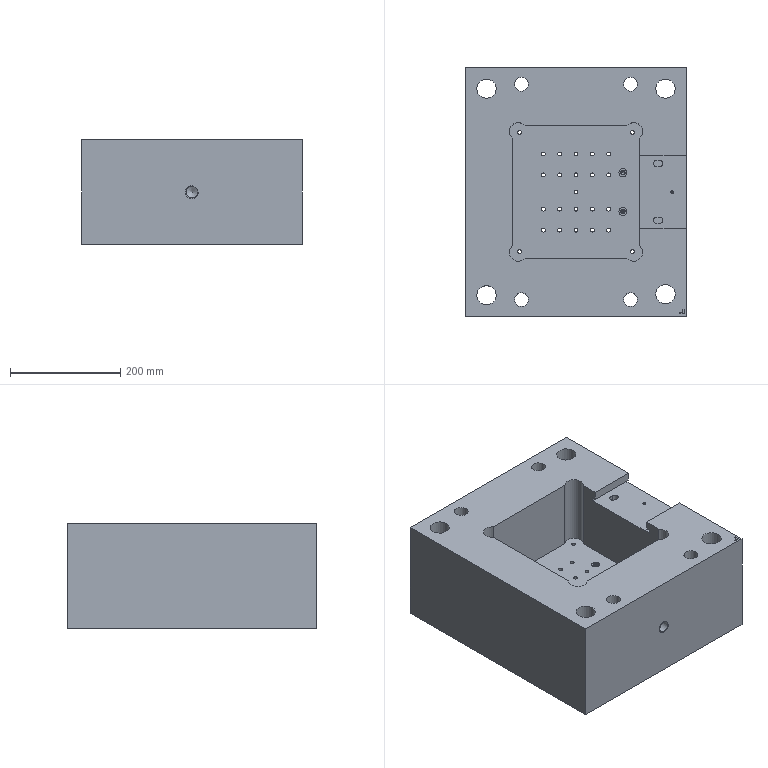Part | NX | features solid 2 | 1 solid | 200 faces | box 400 x 450 x 190 mm | volume 25227574 mm3 | plane 93 | cylinder 90 | cone 17 | commonest cylinder face diameters 7 x25 14.1 x6 15.7 x6 16 x6 6 x4 11 x4